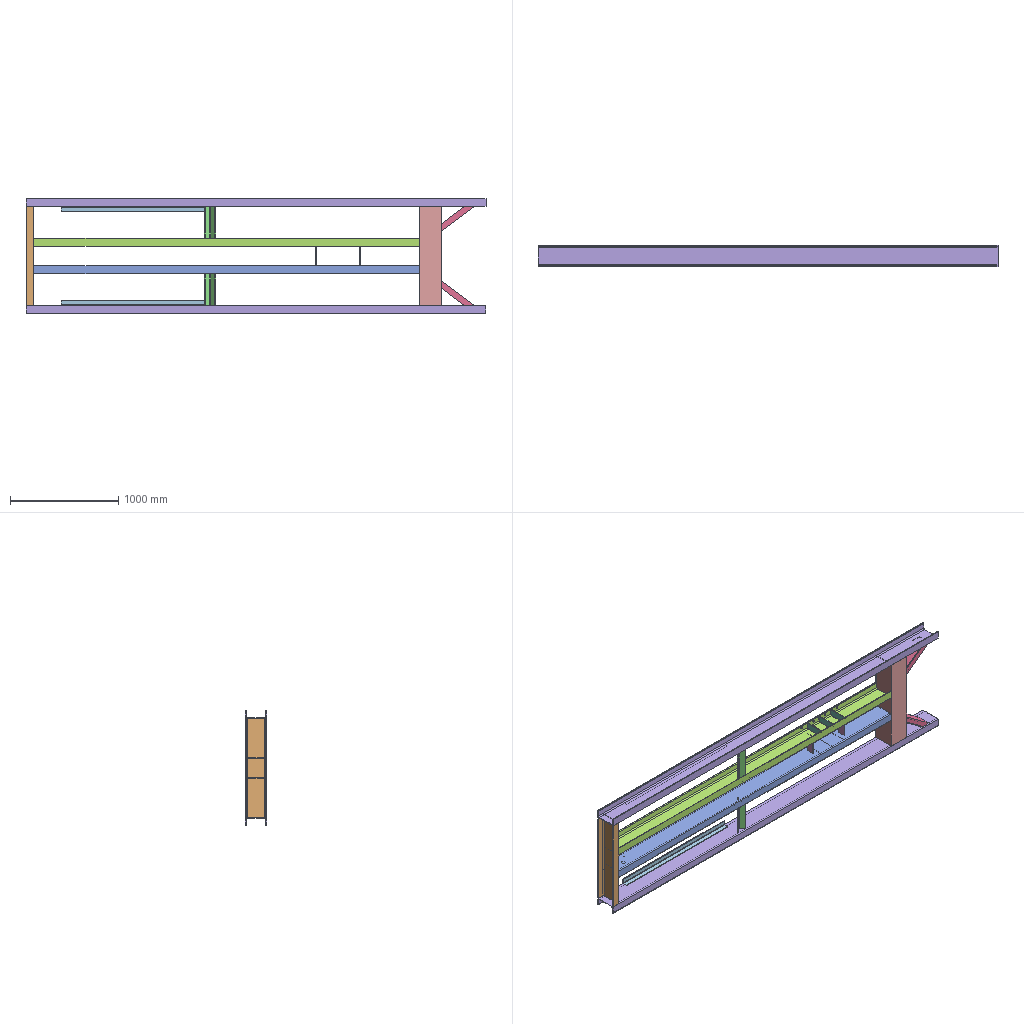Assembly | SolidWorks | 10 different items | 21 placed | box 4242 x 200 x 1060 mm
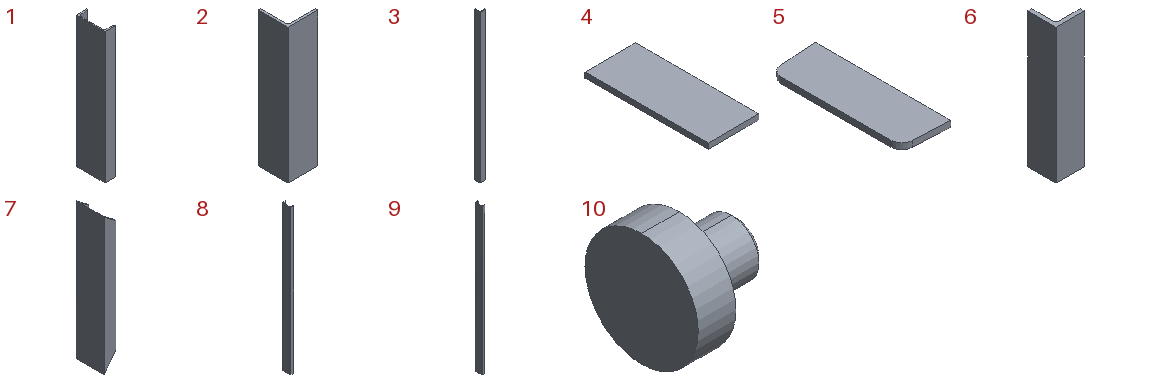Parts list (item | quantity | size | volume | features):
1 | x1 | 73 x 200 x 914.4 mm | 2618794 mm3 | features Extrusion 1
2 | x1 | 200 x 200 x 914.4 mm | 4996450 mm3 | features Extrusion 1
3 | x2 | 50 x 50 x 1321 mm | 751238 mm3 | features Extrusion 1
4 | x2 | 76.2 x 184.2 x 8 mm | 112288 mm3 | features Extrusion 1
5 | x6 | 63.5 x 181.351 x 8 mm | 89849 mm3 | features Extrusion 1
6 | x2 | 75 x 75 x 358.1 mm | 505682 mm3 | features Extrusion 1
7 | x2 | 53 x 126 x 613 mm | 899229 mm3 | features Extrusion 1, ICE 1
8 | x2 | 73 x 200 x 3556 mm | 10184198 mm3 | features Extrusion 1
9 | x2 | 73 x 200 x 4242 mm | 12148294 mm3 | features Extrusion 1
10 | x1 | 31.75 x 38.1 x 38.1 mm | 19559 mm3 | features Revolution 1
Mates (type | each side: item.copy, entity, surface, feature):
Coincident | 2.1 face plane Boss-Extrude1 | 8.1 face plane | 2 times
DistanceDim | 8.1 face plane | assembly plane
Coincident | 4.1 plane | assembly plane
DistanceDim | 4.1 face plane Boss-Extrude1 | 2.1 face plane Boss-Extrude1
DistanceDim | 4.1 plane | 8.1 plane
Coincident | 8.2 face plane | 5.1 face plane Boss-Extrude1
DistanceDim | 5.1 plane | 8.2 face plane
DistanceDim | 5.1 face plane Boss-Extrude1 | 2.1 face plane Boss-Extrude1
Coincident | 8.1 face plane | 1.1 face plane Boss-Extrude1 | 2 times
Coincident | 1.1 plane | assembly plane
Coincident | 1.1 face plane Boss-Extrude1 | 9.1 face plane Boss-Extrude1 | 3 times
Coincident | 9.1 face plane Boss-Extrude1 | 6.1 face plane Boss-Extrude1
PlanarAngleDim | 6.1 face plane Boss-Extrude1 | 9.1 face plane Boss-Extrude1
DistanceDim | 6.1 edge | 9.1 face plane Boss-Extrude1
DistanceDim | 6.1 edge | 2.1 face plane Boss-Extrude1
Coincident | 2.1 face plane Boss-Extrude1 | 7.1 face plane Cut-Extrude1
Coincident | 8.1 face plane | 7.1 edge
Coincident | 2.1 face plane Boss-Extrude1 | 7.1 face plane Boss-Extrude1
Coincident | 9.1 face plane Boss-Extrude1 | 3.1 face plane Boss-Extrude1 | 2 times
DistanceDim | 1.1 face plane Boss-Extrude1 | 3.1 face plane Boss-Extrude1
Coincident | 8.1 face plane | 10.1 edge
DistanceDim | 10.1 plane | 8.1 face plane
DistanceDim | 10.1 plane | 1.1 face plane Boss-Extrude1